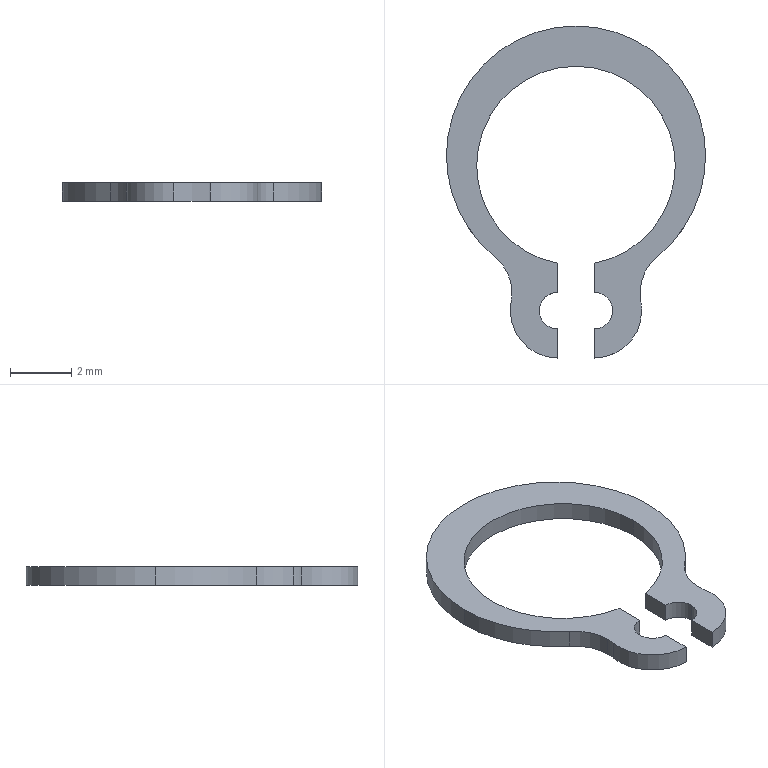Part | STEP file | 1 solid | 21 faces | box 8.48 x 10.864 x 0.6 mm | volume 17.151 mm3 | cylinder 15 | plane 6 | commonest cylinder face diameters 3.1 x6 1.2 x3 6.5 x3 8.48 x3